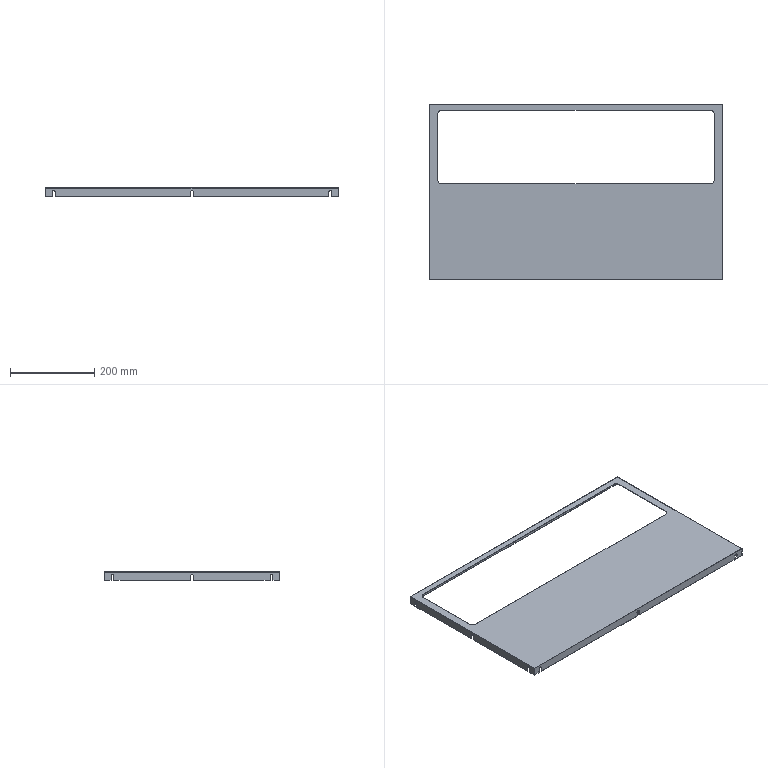Part | STEP file | PN_0003 | 1 solid | 72 faces | box 698 x 418 x 20 mm | volume 217961 mm3 | plane 50 | cylinder 22 | commonest cylinder face diameters 7 x18 20 x4